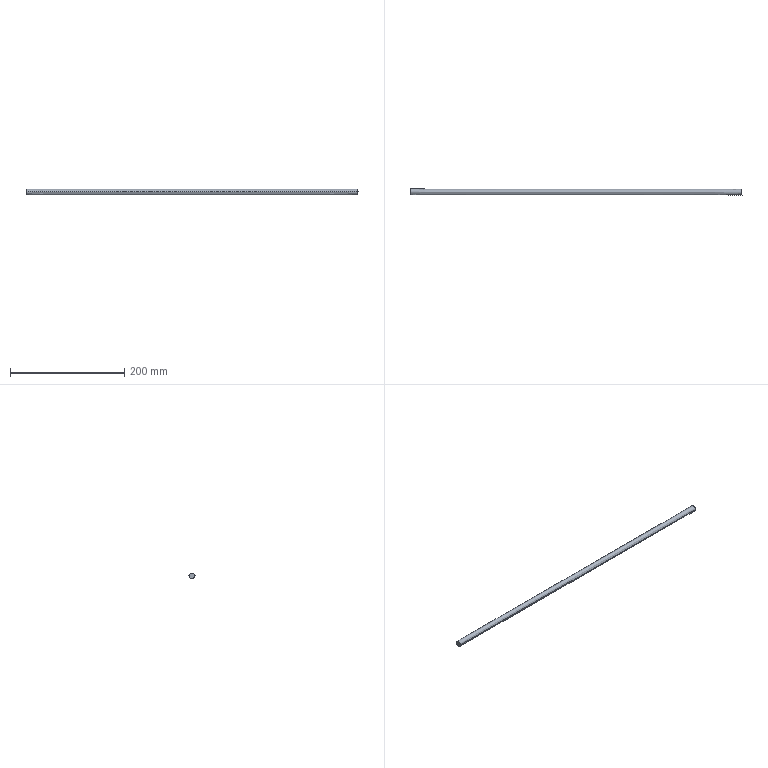Part | NX | features BREP 1 | 1 solid | 4 faces | box 581.307 x 10.561 x 10 mm | volume 45569 mm3 | spline 2 | plane 2
STEP:
#1=CARTESIAN_POINT('',(-525.213,111.233,217.465));
#2=VERTEX_POINT('',#1);
#3=CARTESIAN_POINT('',(56.08,110.678,217.465));
#4=VERTEX_POINT('',#3);
#5=CARTESIAN_POINT('',(-525.213,111.233,217.465));
#6=CARTESIAN_POINT('',(-512.605,111.218,217.465));
#7=CARTESIAN_POINT('',(-487.343,111.188,217.465));
#8=CARTESIAN_POINT('',(-447.77,111.141,217.465));
#9=CARTESIAN_POINT('',(-406.333,111.091,217.465));
#10=CARTESIAN_POINT('',(-363.74,111.038,217.465));
#11=CARTESIAN_POINT('',(-321.148,110.983,217.465));
#12=CARTESIAN_POINT('',(-279.712,110.928,217.465));
#13=CARTESIAN_POINT('',(-240.135,110.875,217.465));
#14=CARTESIAN_POINT('',(-204.166,110.826,217.465));
#15=CARTESIAN_POINT('',(-170.163,110.783,217.465));
#16=CARTESIAN_POINT('',(-127.181,110.734,217.465));
#17=CARTESIAN_POINT('',(-73.095,110.687,217.465));
#18=CARTESIAN_POINT('',(-8.179,110.667,217.465));
#19=CARTESIAN_POINT('',(34.677,110.675,217.465));
#20=CARTESIAN_POINT('',(56.08,110.678,217.465));
#21=B_SPLINE_CURVE_WITH_KNOTS('',3,(#5,#6,#7,#8,#9,#10,#11,#12,#13,#14,#15,#16,#17,#18,#19,#20),.UNSPECIFIED.,.F.,.F.,(4,1,1,1,1,1,1,1,1,1,1,1,1,4),(0.,0.06761,0.1352,0.2028,0.2704,0.3381,0.4057,0.4733,0.5409,0.5983,0.6557,0.7704,0.8852,1.),.UNSPECIFIED.);
#22=EDGE_CURVE('',#2,#4,#21,.T.);
#23=ORIENTED_EDGE('',*,*,#22,.F.);
#24=CARTESIAN_POINT('',(-525.225,101.233,217.465));
#25=VERTEX_POINT('',#24);
#26=CARTESIAN_POINT('',(-525.213,111.233,217.465));
#27=CARTESIAN_POINT('',(-525.213,111.233,218.644));
#28=CARTESIAN_POINT('',(-525.214,110.339,221.221));
#29=CARTESIAN_POINT('',(-525.219,106.233,223.087));
#30=CARTESIAN_POINT('',(-525.224,102.127,221.221));
#31=CARTESIAN_POINT('',(-525.225,101.233,218.644));
#32=CARTESIAN_POINT('',(-525.225,101.233,217.465));
#33=B_SPLINE_CURVE_WITH_KNOTS('',3,(#26,#27,#28,#29,#30,#31,#32),.UNSPECIFIED.,.F.,.F.,(4,1,1,1,4),(0.,0.25,0.5,0.75,1.),.UNSPECIFIED.);
#34=EDGE_CURVE('',#2,#25,#33,.T.);
#35=ORIENTED_EDGE('',*,*,#34,.T.);
#36=CARTESIAN_POINT('',(56.082,100.678,217.465));
#37=VERTEX_POINT('',#36);
#38=CARTESIAN_POINT('',(-525.225,101.233,217.465));
#39=CARTESIAN_POINT('',(-512.617,101.218,217.465));
#40=CARTESIAN_POINT('',(-487.355,101.188,217.465));
#41=CARTESIAN_POINT('',(-447.782,101.141,217.465));
#42=CARTESIAN_POINT('',(-406.345,101.091,217.465));
#43=CARTESIAN_POINT('',(-363.753,101.038,217.465));
#44=CARTESIAN_POINT('',(-321.161,100.983,217.465));
#45=CARTESIAN_POINT('',(-279.726,100.928,217.465));
#46=CARTESIAN_POINT('',(-240.148,100.875,217.465));
#47=CARTESIAN_POINT('',(-204.179,100.826,217.465));
#48=CARTESIAN_POINT('',(-170.175,100.783,217.465));
#49=CARTESIAN_POINT('',(-127.192,100.734,217.465));
#50=CARTESIAN_POINT('',(-73.103,100.687,217.465));
#51=CARTESIAN_POINT('',(-8.182,100.667,217.465));
#52=CARTESIAN_POINT('',(34.679,100.675,217.465));
#53=CARTESIAN_POINT('',(56.082,100.678,217.465));
#54=B_SPLINE_CURVE_WITH_KNOTS('',3,(#38,#39,#40,#41,#42,#43,#44,#45,#46,#47,#48,#49,#50,#51,#52,#53),.UNSPECIFIED.,.F.,.F.,(4,1,1,1,1,1,1,1,1,1,1,1,1,4),(0.,0.06761,0.1352,0.2028,0.2704,0.3381,0.4057,0.4733,0.5409,0.5983,0.6557,0.7704,0.8852,1.),.UNSPECIFIED.);
#55=EDGE_CURVE('',#25,#37,#54,.T.);
#56=ORIENTED_EDGE('',*,*,#55,.T.);
#57=CARTESIAN_POINT('',(56.08,110.678,217.465));
#58=CARTESIAN_POINT('',(56.08,110.678,218.644));
#59=CARTESIAN_POINT('',(56.08,109.784,221.221));
#60=CARTESIAN_POINT('',(56.081,105.678,223.087));
#61=CARTESIAN_POINT('',(56.082,101.572,221.221));
#62=CARTESIAN_POINT('',(56.082,100.678,218.644));
#63=CARTESIAN_POINT('',(56.082,100.678,217.465));
#64=B_SPLINE_CURVE_WITH_KNOTS('',3,(#57,#58,#59,#60,#61,#62,#63),.UNSPECIFIED.,.F.,.F.,(4,1,1,1,4),(0.,0.25,0.5,0.75,1.),.UNSPECIFIED.);
#65=EDGE_CURVE('',#4,#37,#64,.T.);
#66=ORIENTED_EDGE('',*,*,#65,.F.);
#67=EDGE_LOOP('',(#23,#35,#56,#66));
#68=FACE_BOUND('',#67,.T.);
#69=CARTESIAN_POINT('',(-525.225,101.233,217.465));
#70=CARTESIAN_POINT('',(-525.225,101.233,218.644));
#71=CARTESIAN_POINT('',(-525.224,102.127,221.221));
#72=CARTESIAN_POINT('',(-525.219,106.233,223.087));
#73=CARTESIAN_POINT('',(-525.214,110.339,221.221));
#74=CARTESIAN_POINT('',(-525.213,111.233,218.644));
#75=CARTESIAN_POINT('',(-525.213,111.233,217.465));
#76=CARTESIAN_POINT('',(-512.617,101.218,217.465));
#77=CARTESIAN_POINT('',(-512.617,101.218,218.643));
#78=CARTESIAN_POINT('',(-512.616,102.112,221.221));
#79=CARTESIAN_POINT('',(-512.611,106.218,223.087));
#80=CARTESIAN_POINT('',(-512.606,110.324,221.221));
#81=CARTESIAN_POINT('',(-512.605,111.218,218.643));
#82=CARTESIAN_POINT('',(-512.605,111.218,217.465));
#83=CARTESIAN_POINT('',(-487.355,101.188,217.465));
#84=CARTESIAN_POINT('',(-487.355,101.188,218.643));
#85=CARTESIAN_POINT('',(-487.354,102.082,221.221));
#86=CARTESIAN_POINT('',(-487.349,106.188,223.087));
#87=CARTESIAN_POINT('',(-487.344,110.294,221.221));
#88=CARTESIAN_POINT('',(-487.343,111.188,218.643));
#89=CARTESIAN_POINT('',(-487.343,111.188,217.465));
#90=CARTESIAN_POINT('',(-447.782,101.141,217.465));
#91=CARTESIAN_POINT('',(-447.782,101.141,218.643));
#92=CARTESIAN_POINT('',(-447.781,102.035,221.22));
#93=CARTESIAN_POINT('',(-447.776,106.141,223.087));
#94=CARTESIAN_POINT('',(-447.771,110.247,221.22));
#95=CARTESIAN_POINT('',(-447.77,111.141,218.643));
#96=CARTESIAN_POINT('',(-447.77,111.141,217.465));
#97=CARTESIAN_POINT('',(-406.345,101.091,217.465));
#98=CARTESIAN_POINT('',(-406.345,101.091,218.643));
#99=CARTESIAN_POINT('',(-406.344,101.985,221.221));
#100=CARTESIAN_POINT('',(-406.339,106.091,223.087));
#101=CARTESIAN_POINT('',(-406.334,110.197,221.221));
#102=CARTESIAN_POINT('',(-406.333,111.091,218.643));
#103=CARTESIAN_POINT('',(-406.333,111.091,217.465));
#104=CARTESIAN_POINT('',(-363.753,101.038,217.465));
#105=CARTESIAN_POINT('',(-363.753,101.038,218.643));
#106=CARTESIAN_POINT('',(-363.752,101.932,221.221));
#107=CARTESIAN_POINT('',(-363.747,106.038,223.087));
#108=CARTESIAN_POINT('',(-363.741,110.144,221.221));
#109=CARTESIAN_POINT('',(-363.74,111.038,218.643));
#110=CARTESIAN_POINT('',(-363.74,111.038,217.465));
#111=CARTESIAN_POINT('',(-321.161,100.983,217.465));
#112=CARTESIAN_POINT('',(-321.161,100.983,218.643));
#113=CARTESIAN_POINT('',(-321.16,101.878,221.221));
#114=CARTESIAN_POINT('',(-321.154,105.983,223.087));
#115=CARTESIAN_POINT('',(-321.149,110.089,221.221));
#116=CARTESIAN_POINT('',(-321.148,110.983,218.643));
#117=CARTESIAN_POINT('',(-321.148,110.983,217.465));
#118=CARTESIAN_POINT('',(-279.726,100.928,217.465));
#119=CARTESIAN_POINT('',(-279.726,100.928,218.644));
#120=CARTESIAN_POINT('',(-279.724,101.823,221.221));
#121=CARTESIAN_POINT('',(-279.719,105.928,223.087));
#122=CARTESIAN_POINT('',(-279.713,110.034,221.221));
#123=CARTESIAN_POINT('',(-279.712,110.928,218.644));
#124=CARTESIAN_POINT('',(-279.712,110.928,217.465));
#125=CARTESIAN_POINT('',(-240.148,100.875,217.465));
#126=CARTESIAN_POINT('',(-240.148,100.875,218.643));
#127=CARTESIAN_POINT('',(-240.147,101.769,221.221));
#128=CARTESIAN_POINT('',(-240.141,105.875,223.087));
#129=CARTESIAN_POINT('',(-240.136,109.981,221.221));
#130=CARTESIAN_POINT('',(-240.135,110.875,218.643));
#131=CARTESIAN_POINT('',(-240.135,110.875,217.465));
#132=CARTESIAN_POINT('',(-204.179,100.826,217.465));
#133=CARTESIAN_POINT('',(-204.179,100.826,218.643));
#134=CARTESIAN_POINT('',(-204.178,101.721,221.221));
#135=CARTESIAN_POINT('',(-204.172,105.826,223.087));
#136=CARTESIAN_POINT('',(-204.167,109.932,221.221));
#137=CARTESIAN_POINT('',(-204.166,110.826,218.643));
#138=CARTESIAN_POINT('',(-204.166,110.826,217.465));
#139=CARTESIAN_POINT('',(-170.175,100.783,217.465));
#140=CARTESIAN_POINT('',(-170.175,100.783,218.643));
#141=CARTESIAN_POINT('',(-170.174,101.678,221.221));
#142=CARTESIAN_POINT('',(-170.169,105.783,223.087));
#143=CARTESIAN_POINT('',(-170.164,109.889,221.221));
#144=CARTESIAN_POINT('',(-170.163,110.783,218.643));
#145=CARTESIAN_POINT('',(-170.163,110.783,217.465));
#146=CARTESIAN_POINT('',(-127.192,100.734,217.465));
#147=CARTESIAN_POINT('',(-127.192,100.734,218.643));
#148=CARTESIAN_POINT('',(-127.191,101.628,221.221));
#149=CARTESIAN_POINT('',(-127.186,105.734,223.087));
#150=CARTESIAN_POINT('',(-127.182,109.84,221.221));
#151=CARTESIAN_POINT('',(-127.181,110.734,218.643));
#152=CARTESIAN_POINT('',(-127.181,110.734,217.465));
#153=CARTESIAN_POINT('',(-73.103,100.687,217.465));
#154=CARTESIAN_POINT('',(-73.103,100.687,218.643));
#155=CARTESIAN_POINT('',(-73.103,101.581,221.221));
#156=CARTESIAN_POINT('',(-73.099,105.687,223.087));
#157=CARTESIAN_POINT('',(-73.096,109.793,221.221));
#158=CARTESIAN_POINT('',(-73.095,110.687,218.643));
#159=CARTESIAN_POINT('',(-73.095,110.687,217.465));
#160=CARTESIAN_POINT('',(-8.182,100.667,217.465));
#161=CARTESIAN_POINT('',(-8.182,100.667,218.644));
#162=CARTESIAN_POINT('',(-8.181,101.561,221.221));
#163=CARTESIAN_POINT('',(-8.18,105.667,223.087));
#164=CARTESIAN_POINT('',(-8.179,109.772,221.221));
#165=CARTESIAN_POINT('',(-8.179,110.667,218.644));
#166=CARTESIAN_POINT('',(-8.179,110.667,217.465));
#167=CARTESIAN_POINT('',(34.679,100.675,217.465));
#168=CARTESIAN_POINT('',(34.679,100.675,218.644));
#169=CARTESIAN_POINT('',(34.679,101.569,221.221));
#170=CARTESIAN_POINT('',(34.678,105.675,223.087));
#171=CARTESIAN_POINT('',(34.677,109.781,221.221));
#172=CARTESIAN_POINT('',(34.677,110.675,218.644));
#173=CARTESIAN_POINT('',(34.677,110.675,217.465));
#174=CARTESIAN_POINT('',(56.082,100.678,217.465));
#175=CARTESIAN_POINT('',(56.082,100.678,218.644));
#176=CARTESIAN_POINT('',(56.082,101.572,221.221));
#177=CARTESIAN_POINT('',(56.081,105.678,223.087));
#178=CARTESIAN_POINT('',(56.08,109.784,221.221));
#179=CARTESIAN_POINT('',(56.08,110.678,218.644));
#180=CARTESIAN_POINT('',(56.08,110.678,217.465));
#181=B_SPLINE_SURFACE_WITH_KNOTS('',3,3,((#69,#70,#71,#72,#73,#74,#75),(#76,#77,#78,#79,#80,#81,#82),(#83,#84,#85,#86,#87,#88,#89),(#90,#91,#92,#93,#94,#95,#96),(#97,#98,#99,#100,#101,#102,#103),(#104,#105,#106,#107,#108,#109,#110),(#111,#112,#113,#114,#115,#116,#117),(#118,#119,#120,#121,#122,#123,#124),(#125,#126,#127,#128,#129,#130,#131),(#132,#133,#134,#135,#136,#137,#138),(#139,#140,#141,#142,#143,#144,#145),(#146,#147,#148,#149,#150,#151,#152),(#153,#154,#155,#156,#157,#158,#159),(#160,#161,#162,#163,#164,#165,#166),(#167,#168,#169,#170,#171,#172,#173),(#174,#175,#176,#177,#178,#179,#180)),.UNSPECIFIED.,.F.,.F.,.F.,(4,1,1,1,1,1,1,1,1,1,1,1,1,4),(4,1,1,1,4),(0.01018,0.07642,0.1427,0.2089,0.2751,0.3414,0.4076,0.4738,0.5401,0.5963,0.6525,0.7649,0.8774,0.9898),(0.02629,0.2633,0.5003,0.7373,0.9742),.UNSPECIFIED.);
#182=ADVANCED_FACE('',(#68),#181,.T.);
#183=ORIENTED_EDGE('',*,*,#55,.F.);
#184=CARTESIAN_POINT('',(-525.225,101.233,217.465));
#185=CARTESIAN_POINT('',(-525.225,101.233,216.286));
#186=CARTESIAN_POINT('',(-525.224,102.127,213.709));
#187=CARTESIAN_POINT('',(-525.219,106.233,211.843));
#188=CARTESIAN_POINT('',(-525.214,110.339,213.709));
#189=CARTESIAN_POINT('',(-525.213,111.233,216.286));
#190=CARTESIAN_POINT('',(-525.213,111.233,217.465));
#191=B_SPLINE_CURVE_WITH_KNOTS('',3,(#184,#185,#186,#187,#188,#189,#190),.UNSPECIFIED.,.F.,.F.,(4,1,1,1,4),(0.,0.25,0.5,0.75,1.),.UNSPECIFIED.);
#192=EDGE_CURVE('',#25,#2,#191,.T.);
#193=ORIENTED_EDGE('',*,*,#192,.T.);
#194=ORIENTED_EDGE('',*,*,#22,.T.);
#195=CARTESIAN_POINT('',(56.082,100.678,217.465));
#196=CARTESIAN_POINT('',(56.082,100.678,216.286));
#197=CARTESIAN_POINT('',(56.082,101.572,213.709));
#198=CARTESIAN_POINT('',(56.081,105.678,211.843));
#199=CARTESIAN_POINT('',(56.08,109.784,213.709));
#200=CARTESIAN_POINT('',(56.08,110.678,216.286));
#201=CARTESIAN_POINT('',(56.08,110.678,217.465));
#202=B_SPLINE_CURVE_WITH_KNOTS('',3,(#195,#196,#197,#198,#199,#200,#201),.UNSPECIFIED.,.F.,.F.,(4,1,1,1,4),(0.,0.25,0.5,0.75,1.),.UNSPECIFIED.);
#203=EDGE_CURVE('',#37,#4,#202,.T.);
#204=ORIENTED_EDGE('',*,*,#203,.F.);
#205=EDGE_LOOP('',(#183,#193,#194,#204));
#206=FACE_BOUND('',#205,.T.);
#207=CARTESIAN_POINT('',(-525.213,111.233,217.465));
#208=CARTESIAN_POINT('',(-525.213,111.233,216.286));
#209=CARTESIAN_POINT('',(-525.214,110.339,213.709));
#210=CARTESIAN_POINT('',(-525.219,106.233,211.843));
#211=CARTESIAN_POINT('',(-525.224,102.127,213.709));
#212=CARTESIAN_POINT('',(-525.225,101.233,216.286));
#213=CARTESIAN_POINT('',(-525.225,101.233,217.465));
#214=CARTESIAN_POINT('',(-512.605,111.218,217.465));
#215=CARTESIAN_POINT('',(-512.605,111.218,216.286));
#216=CARTESIAN_POINT('',(-512.606,110.324,213.709));
#217=CARTESIAN_POINT('',(-512.611,106.218,211.843));
#218=CARTESIAN_POINT('',(-512.616,102.112,213.709));
#219=CARTESIAN_POINT('',(-512.617,101.218,216.286));
#220=CARTESIAN_POINT('',(-512.617,101.218,217.465));
#221=CARTESIAN_POINT('',(-487.343,111.188,217.465));
#222=CARTESIAN_POINT('',(-487.343,111.188,216.286));
#223=CARTESIAN_POINT('',(-487.344,110.294,213.709));
#224=CARTESIAN_POINT('',(-487.349,106.188,211.843));
#225=CARTESIAN_POINT('',(-487.354,102.082,213.709));
#226=CARTESIAN_POINT('',(-487.355,101.188,216.286));
#227=CARTESIAN_POINT('',(-487.355,101.188,217.465));
#228=CARTESIAN_POINT('',(-447.77,111.141,217.465));
#229=CARTESIAN_POINT('',(-447.77,111.141,216.286));
#230=CARTESIAN_POINT('',(-447.771,110.247,213.709));
#231=CARTESIAN_POINT('',(-447.776,106.141,211.843));
#232=CARTESIAN_POINT('',(-447.781,102.035,213.709));
#233=CARTESIAN_POINT('',(-447.782,101.141,216.286));
#234=CARTESIAN_POINT('',(-447.782,101.141,217.465));
#235=CARTESIAN_POINT('',(-406.333,111.091,217.465));
#236=CARTESIAN_POINT('',(-406.333,111.091,216.286));
#237=CARTESIAN_POINT('',(-406.334,110.197,213.709));
#238=CARTESIAN_POINT('',(-406.339,106.091,211.843));
#239=CARTESIAN_POINT('',(-406.344,101.985,213.709));
#240=CARTESIAN_POINT('',(-406.345,101.091,216.286));
#241=CARTESIAN_POINT('',(-406.345,101.091,217.465));
#242=CARTESIAN_POINT('',(-363.74,111.038,217.465));
#243=CARTESIAN_POINT('',(-363.74,111.038,216.286));
#244=CARTESIAN_POINT('',(-363.742,110.144,213.709));
#245=CARTESIAN_POINT('',(-363.747,106.038,211.843));
#246=CARTESIAN_POINT('',(-363.752,101.932,213.709));
#247=CARTESIAN_POINT('',(-363.753,101.038,216.286));
#248=CARTESIAN_POINT('',(-363.753,101.038,217.465));
#249=CARTESIAN_POINT('',(-321.148,110.983,217.465));
#250=CARTESIAN_POINT('',(-321.148,110.983,216.286));
#251=CARTESIAN_POINT('',(-321.149,110.089,213.709));
#252=CARTESIAN_POINT('',(-321.154,105.983,211.843));
#253=CARTESIAN_POINT('',(-321.16,101.878,213.709));
#254=CARTESIAN_POINT('',(-321.161,100.983,216.286));
#255=CARTESIAN_POINT('',(-321.161,100.983,217.465));
#256=CARTESIAN_POINT('',(-279.712,110.928,217.465));
#257=CARTESIAN_POINT('',(-279.712,110.928,216.286));
#258=CARTESIAN_POINT('',(-279.713,110.034,213.709));
#259=CARTESIAN_POINT('',(-279.719,105.928,211.843));
#260=CARTESIAN_POINT('',(-279.724,101.823,213.709));
#261=CARTESIAN_POINT('',(-279.726,100.928,216.286));
#262=CARTESIAN_POINT('',(-279.726,100.928,217.465));
#263=CARTESIAN_POINT('',(-240.135,110.875,217.465));
#264=CARTESIAN_POINT('',(-240.135,110.875,216.286));
#265=CARTESIAN_POINT('',(-240.136,109.981,213.709));
#266=CARTESIAN_POINT('',(-240.141,105.875,211.843));
#267=CARTESIAN_POINT('',(-240.147,101.769,213.709));
#268=CARTESIAN_POINT('',(-240.148,100.875,216.286));
#269=CARTESIAN_POINT('',(-240.148,100.875,217.465));
#270=CARTESIAN_POINT('',(-204.166,110.826,217.465));
#271=CARTESIAN_POINT('',(-204.166,110.826,216.286));
#272=CARTESIAN_POINT('',(-204.167,109.932,213.709));
#273=CARTESIAN_POINT('',(-204.172,105.826,211.843));
#274=CARTESIAN_POINT('',(-204.178,101.721,213.709));
#275=CARTESIAN_POINT('',(-204.179,100.826,216.286));
#276=CARTESIAN_POINT('',(-204.179,100.826,217.465));
#277=CARTESIAN_POINT('',(-170.163,110.783,217.465));
#278=CARTESIAN_POINT('',(-170.163,110.783,216.286));
#279=CARTESIAN_POINT('',(-170.164,109.889,213.709));
#280=CARTESIAN_POINT('',(-170.169,105.783,211.843));
#281=CARTESIAN_POINT('',(-170.174,101.678,213.709));
#282=CARTESIAN_POINT('',(-170.175,100.783,216.286));
#283=CARTESIAN_POINT('',(-170.175,100.783,217.465));
#284=CARTESIAN_POINT('',(-127.181,110.734,217.465));
#285=CARTESIAN_POINT('',(-127.181,110.734,216.286));
#286=CARTESIAN_POINT('',(-127.182,109.84,213.709));
#287=CARTESIAN_POINT('',(-127.186,105.734,211.843));
#288=CARTESIAN_POINT('',(-127.191,101.628,213.709));
#289=CARTESIAN_POINT('',(-127.192,100.734,216.286));
#290=CARTESIAN_POINT('',(-127.192,100.734,217.465));
#291=CARTESIAN_POINT('',(-73.095,110.687,217.465));
#292=CARTESIAN_POINT('',(-73.095,110.687,216.286));
#293=CARTESIAN_POINT('',(-73.096,109.793,213.709));
#294=CARTESIAN_POINT('',(-73.099,105.687,211.843));
#295=CARTESIAN_POINT('',(-73.103,101.581,213.709));
#296=CARTESIAN_POINT('',(-73.103,100.687,216.286));
#297=CARTESIAN_POINT('',(-73.103,100.687,217.465));
#298=CARTESIAN_POINT('',(-8.179,110.667,217.465));
#299=CARTESIAN_POINT('',(-8.179,110.667,216.286));
#300=CARTESIAN_POINT('',(-8.179,109.772,213.709));
#301=CARTESIAN_POINT('',(-8.18,105.667,211.843));
#302=CARTESIAN_POINT('',(-8.181,101.561,213.709));
#303=CARTESIAN_POINT('',(-8.182,100.667,216.286));
#304=CARTESIAN_POINT('',(-8.182,100.667,217.465));
#305=CARTESIAN_POINT('',(34.677,110.675,217.465));
#306=CARTESIAN_POINT('',(34.677,110.675,216.286));
#307=CARTESIAN_POINT('',(34.677,109.781,213.709));
#308=CARTESIAN_POINT('',(34.678,105.675,211.843));
#309=CARTESIAN_POINT('',(34.679,101.569,213.709));
#310=CARTESIAN_POINT('',(34.679,100.675,216.286));
#311=CARTESIAN_POINT('',(34.679,100.675,217.465));
#312=CARTESIAN_POINT('',(56.08,110.678,217.465));
#313=CARTESIAN_POINT('',(56.08,110.678,216.286));
#314=CARTESIAN_POINT('',(56.08,109.784,213.709));
#315=CARTESIAN_POINT('',(56.081,105.678,211.843));
#316=CARTESIAN_POINT('',(56.082,101.572,213.709));
#317=CARTESIAN_POINT('',(56.082,100.678,216.286));
#318=CARTESIAN_POINT('',(56.082,100.678,217.465));
#319=B_SPLINE_SURFACE_WITH_KNOTS('',3,3,((#207,#208,#209,#210,#211,#212,#213),(#214,#215,#216,#217,#218,#219,#220),(#221,#222,#223,#224,#225,#226,#227),(#228,#229,#230,#231,#232,#233,#234),(#235,#236,#237,#238,#239,#240,#241),(#242,#243,#244,#245,#246,#247,#248),(#249,#250,#251,#252,#253,#254,#255),(#256,#257,#258,#259,#260,#261,#262),(#263,#264,#265,#266,#267,#268,#269),(#270,#271,#272,#273,#274,#275,#276),(#277,#278,#279,#280,#281,#282,#283),(#284,#285,#286,#287,#288,#289,#290),(#291,#292,#293,#294,#295,#296,#297),(#298,#299,#300,#301,#302,#303,#304),(#305,#306,#307,#308,#309,#310,#311),(#312,#313,#314,#315,#316,#317,#318)),.UNSPECIFIED.,.F.,.F.,.F.,(4,1,1,1,1,1,1,1,1,1,1,1,1,4),(4,1,1,1,4),(0.01018,0.07642,0.1427,0.2089,0.2751,0.3414,0.4076,0.4738,0.5401,0.5963,0.6525,0.7649,0.8774,0.9898),(0.02629,0.2633,0.5003,0.7373,0.9742),.UNSPECIFIED.);
#320=ADVANCED_FACE('',(#206),#319,.T.);
#321=ORIENTED_EDGE('',*,*,#34,.F.);
#322=ORIENTED_EDGE('',*,*,#192,.F.);
#323=EDGE_LOOP('',(#321,#322));
#324=FACE_BOUND('',#323,.T.);
#325=CARTESIAN_POINT('',(-525.213,111.233,217.465));
#326=DIRECTION('',(-1.,0.001187,0.000005612));
#327=DIRECTION('',(-0.000005612,0.,-1.));
#328=AXIS2_PLACEMENT_3D('',#325,#326,#327);
#329=PLANE('',#328);
#330=ADVANCED_FACE('',(#324),#329,.T.);
#331=ORIENTED_EDGE('',*,*,#203,.T.);
#332=ORIENTED_EDGE('',*,*,#65,.T.);
#333=EDGE_LOOP('',(#331,#332));
#334=FACE_BOUND('',#333,.T.);
#335=CARTESIAN_POINT('',(56.08,110.678,217.465));
#336=DIRECTION('',(-1.,-0.0001509,0.000000288));
#337=DIRECTION('',(0.0001509,-1.,0.));
#338=AXIS2_PLACEMENT_3D('',#335,#336,#337);
#339=PLANE('',#338);
#340=ADVANCED_FACE('',(#334),#339,.F.);
#341=CLOSED_SHELL('',(#182,#320,#330,#340));
#342=MANIFOLD_SOLID_BREP('',#341);
#343=(LENGTH_UNIT()NAMED_UNIT(*)SI_UNIT(.MILLI.,.METRE.));
#344=UNCERTAINTY_MEASURE_WITH_UNIT(LENGTH_MEASURE(0.00001),#343,'','');
#345=(NAMED_UNIT(*)PLANE_ANGLE_UNIT()SI_UNIT($,.RADIAN.));
#346=(NAMED_UNIT(*)SI_UNIT($,.STERADIAN.)SOLID_ANGLE_UNIT());
#347=(GEOMETRIC_REPRESENTATION_CONTEXT(3)GLOBAL_UNCERTAINTY_ASSIGNED_CONTEXT((#344))GLOBAL_UNIT_ASSIGNED_CONTEXT((#343,#345,#346))REPRESENTATION_CONTEXT('',''));
#348=ADVANCED_BREP_SHAPE_REPRESENTATION('',(#342),#347);